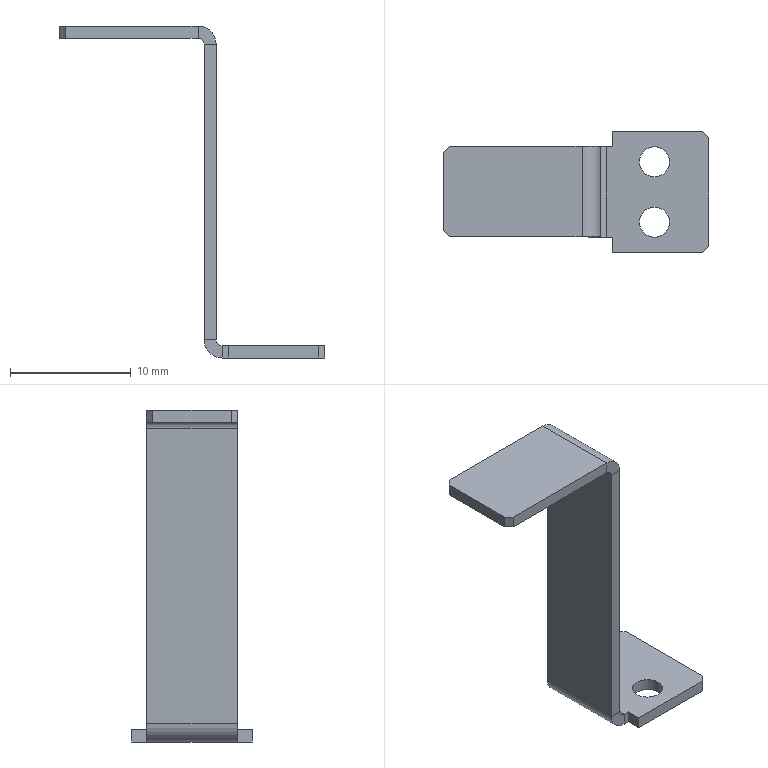Part | NX | 1 solid | 32 faces | box 22 x 10 x 27.5 mm | volume 366.994 mm3 | plane 26 | cylinder 6 | commonest cylinder face diameters 1 x2 2.5 x2 3 x2
STEP:
#1=CARTESIAN_POINT('',(-1.,3.75,0.5));
#2=VERTEX_POINT('',#1);
#3=CARTESIAN_POINT('',(-1.,3.75,25.));
#4=VERTEX_POINT('',#3);
#5=CARTESIAN_POINT('',(-1.,3.75,0.));
#6=DIRECTION('',(0.,0.,1.));
#7=VECTOR('',#6,1000.);
#8=LINE('',#5,#7);
#9=EDGE_CURVE('',#2,#4,#8,.T.);
#10=ORIENTED_EDGE('',*,*,#9,.T.);
#11=CARTESIAN_POINT('',(0.,3.75,25.));
#12=VERTEX_POINT('',#11);
#13=CARTESIAN_POINT('',(-1.,3.75,25.));
#14=DIRECTION('',(1.,0.,0.));
#15=VECTOR('',#14,1000.);
#16=LINE('',#13,#15);
#17=EDGE_CURVE('',#4,#12,#16,.T.);
#18=ORIENTED_EDGE('',*,*,#17,.T.);
#19=CARTESIAN_POINT('',(0.,3.75,0.5));
#20=VERTEX_POINT('',#19);
#21=CARTESIAN_POINT('',(0.,3.75,0.));
#22=DIRECTION('',(0.,0.,1.));
#23=VECTOR('',#22,1000.);
#24=LINE('',#21,#23);
#25=EDGE_CURVE('',#20,#12,#24,.T.);
#26=ORIENTED_EDGE('',*,*,#25,.F.);
#27=CARTESIAN_POINT('',(0.,3.75,0.5));
#28=DIRECTION('',(-1.,0.,0.));
#29=VECTOR('',#28,1000.);
#30=LINE('',#27,#29);
#31=EDGE_CURVE('',#20,#2,#30,.T.);
#32=ORIENTED_EDGE('',*,*,#31,.T.);
#33=EDGE_LOOP('',(#10,#18,#26,#32));
#34=FACE_BOUND('',#33,.T.);
#35=CARTESIAN_POINT('',(0.5,3.75,-1.));
#36=DIRECTION('',(0.,1.,0.));
#37=DIRECTION('',(0.,0.,1.));
#38=AXIS2_PLACEMENT_3D('',#35,#36,#37);
#39=PLANE('',#38);
#40=ADVANCED_FACE('',(#34),#39,.T.);
#41=CARTESIAN_POINT('',(-1.,-3.75,25.));
#42=VERTEX_POINT('',#41);
#43=CARTESIAN_POINT('',(-1.,3.75,25.));
#44=DIRECTION('',(0.,1.,0.));
#45=VECTOR('',#44,1000.);
#46=LINE('',#43,#45);
#47=EDGE_CURVE('',#4,#42,#46,.F.);
#48=ORIENTED_EDGE('',*,*,#47,.F.);
#49=ORIENTED_EDGE('',*,*,#9,.F.);
#50=CARTESIAN_POINT('',(-1.,-3.75,0.5));
#51=VERTEX_POINT('',#50);
#52=CARTESIAN_POINT('',(-1.,3.75,0.5));
#53=DIRECTION('',(0.,-1.,0.));
#54=VECTOR('',#53,1000.);
#55=LINE('',#52,#54);
#56=EDGE_CURVE('',#2,#51,#55,.T.);
#57=ORIENTED_EDGE('',*,*,#56,.T.);
#58=CARTESIAN_POINT('',(-1.,-3.75,0.));
#59=DIRECTION('',(0.,0.,1.));
#60=VECTOR('',#59,1000.);
#61=LINE('',#58,#60);
#62=EDGE_CURVE('',#51,#42,#61,.T.);
#63=ORIENTED_EDGE('',*,*,#62,.T.);
#64=EDGE_LOOP('',(#48,#49,#57,#63));
#65=FACE_BOUND('',#64,.T.);
#66=CARTESIAN_POINT('',(-1.,3.75,0.));
#67=DIRECTION('',(1.,0.,0.));
#68=DIRECTION('',(0.,0.,-1.));
#69=AXIS2_PLACEMENT_3D('',#66,#67,#68);
#70=PLANE('',#69);
#71=ADVANCED_FACE('',(#65),#70,.F.);
#72=ORIENTED_EDGE('',*,*,#25,.T.);
#73=CARTESIAN_POINT('',(0.,-3.75,25.));
#74=VERTEX_POINT('',#73);
#75=CARTESIAN_POINT('',(0.,3.75,25.));
#76=DIRECTION('',(0.,1.,0.));
#77=VECTOR('',#76,1000.);
#78=LINE('',#75,#77);
#79=EDGE_CURVE('',#12,#74,#78,.F.);
#80=ORIENTED_EDGE('',*,*,#79,.T.);
#81=CARTESIAN_POINT('',(0.,-3.75,0.5));
#82=VERTEX_POINT('',#81);
#83=CARTESIAN_POINT('',(0.,-3.75,0.));
#84=DIRECTION('',(0.,0.,1.));
#85=VECTOR('',#84,1000.);
#86=LINE('',#83,#85);
#87=EDGE_CURVE('',#82,#74,#86,.T.);
#88=ORIENTED_EDGE('',*,*,#87,.F.);
#89=CARTESIAN_POINT('',(0.,3.75,0.5));
#90=DIRECTION('',(0.,-1.,0.));
#91=VECTOR('',#90,1000.);
#92=LINE('',#89,#91);
#93=EDGE_CURVE('',#20,#82,#92,.T.);
#94=ORIENTED_EDGE('',*,*,#93,.F.);
#95=EDGE_LOOP('',(#72,#80,#88,#94));
#96=FACE_BOUND('',#95,.T.);
#97=CARTESIAN_POINT('',(0.,3.75,0.));
#98=DIRECTION('',(1.,0.,0.));
#99=DIRECTION('',(0.,0.,-1.));
#100=AXIS2_PLACEMENT_3D('',#97,#98,#99);
#101=PLANE('',#100);
#102=ADVANCED_FACE('',(#96),#101,.T.);
#103=ORIENTED_EDGE('',*,*,#31,.F.);
#104=CARTESIAN_POINT('',(0.5,3.75,0.));
#105=VERTEX_POINT('',#104);
#106=CARTESIAN_POINT('',(0.5,3.75,0.5));
#107=DIRECTION('',(0.,-1.,0.));
#108=DIRECTION('',(0.,0.,-1.));
#109=AXIS2_PLACEMENT_3D('',#106,#107,#108);
#110=CIRCLE('',#109,0.5);
#111=EDGE_CURVE('',#105,#20,#110,.F.);
#112=ORIENTED_EDGE('',*,*,#111,.F.);
#113=CARTESIAN_POINT('',(0.5,3.75,-1.));
#114=VERTEX_POINT('',#113);
#115=CARTESIAN_POINT('',(0.5,3.75,-1.));
#116=DIRECTION('',(0.,0.,1.));
#117=VECTOR('',#116,1000.);
#118=LINE('',#115,#117);
#119=EDGE_CURVE('',#114,#105,#118,.T.);
#120=ORIENTED_EDGE('',*,*,#119,.F.);
#121=CARTESIAN_POINT('',(0.5,3.75,0.5));
#122=DIRECTION('',(0.,1.,0.));
#123=DIRECTION('',(1.,0.,0.));
#124=AXIS2_PLACEMENT_3D('',#121,#122,#123);
#125=CIRCLE('',#124,1.5);
#126=EDGE_CURVE('',#114,#2,#125,.T.);
#127=ORIENTED_EDGE('',*,*,#126,.T.);
#128=EDGE_LOOP('',(#103,#112,#120,#127));
#129=FACE_BOUND('',#128,.T.);
#130=CARTESIAN_POINT('',(0.,3.75,0.5));
#131=DIRECTION('',(0.,1.,0.));
#132=DIRECTION('',(0.,0.,1.));
#133=AXIS2_PLACEMENT_3D('',#130,#131,#132);
#134=PLANE('',#133);
#135=ADVANCED_FACE('',(#129),#134,.T.);
#136=CARTESIAN_POINT('',(0.5,-3.75,0.));
#137=VERTEX_POINT('',#136);
#138=CARTESIAN_POINT('',(0.5,-3.75,-1.));
#139=VERTEX_POINT('',#138);
#140=CARTESIAN_POINT('',(0.5,-3.75,0.));
#141=DIRECTION('',(0.,0.,-1.));
#142=VECTOR('',#141,1000.);
#143=LINE('',#140,#142);
#144=EDGE_CURVE('',#137,#139,#143,.T.);
#145=ORIENTED_EDGE('',*,*,#144,.F.);
#146=CARTESIAN_POINT('',(0.5,-3.75,0.5));
#147=DIRECTION('',(0.,-1.,0.));
#148=DIRECTION('',(0.,0.,-1.));
#149=AXIS2_PLACEMENT_3D('',#146,#147,#148);
#150=CIRCLE('',#149,0.5);
#151=EDGE_CURVE('',#137,#82,#150,.F.);
#152=ORIENTED_EDGE('',*,*,#151,.T.);
#153=CARTESIAN_POINT('',(-1.,-3.75,0.5));
#154=DIRECTION('',(1.,0.,0.));
#155=VECTOR('',#154,1000.);
#156=LINE('',#153,#155);
#157=EDGE_CURVE('',#51,#82,#156,.T.);
#158=ORIENTED_EDGE('',*,*,#157,.F.);
#159=CARTESIAN_POINT('',(0.5,-3.75,0.5));
#160=DIRECTION('',(0.,1.,0.));
#161=DIRECTION('',(1.,0.,0.));
#162=AXIS2_PLACEMENT_3D('',#159,#160,#161);
#163=CIRCLE('',#162,1.5);
#164=EDGE_CURVE('',#139,#51,#163,.T.);
#165=ORIENTED_EDGE('',*,*,#164,.F.);
#166=EDGE_LOOP('',(#145,#152,#158,#165));
#167=FACE_BOUND('',#166,.T.);
#168=CARTESIAN_POINT('',(0.5,-3.75,0.));
#169=DIRECTION('',(0.,-1.,0.));
#170=DIRECTION('',(0.,0.,-1.));
#171=AXIS2_PLACEMENT_3D('',#168,#169,#170);
#172=PLANE('',#171);
#173=ADVANCED_FACE('',(#167),#172,.T.);
#174=CARTESIAN_POINT('',(1.,-3.75,0.));
#175=VERTEX_POINT('',#174);
#176=CARTESIAN_POINT('',(1.,-3.75,-1.));
#177=VERTEX_POINT('',#176);
#178=CARTESIAN_POINT('',(1.,-3.75,0.5));
#179=DIRECTION('',(0.,0.,-1.));
#180=VECTOR('',#179,1000.);
#181=LINE('',#178,#180);
#182=EDGE_CURVE('',#175,#177,#181,.T.);
#183=ORIENTED_EDGE('',*,*,#182,.F.);
#184=CARTESIAN_POINT('',(9.,-3.75,0.));
#185=DIRECTION('',(-1.,0.,0.));
#186=VECTOR('',#185,1000.);
#187=LINE('',#184,#186);
#188=EDGE_CURVE('',#175,#137,#187,.T.);
#189=ORIENTED_EDGE('',*,*,#188,.T.);
#190=ORIENTED_EDGE('',*,*,#144,.T.);
#191=CARTESIAN_POINT('',(9.,-3.75,-1.));
#192=DIRECTION('',(-1.,0.,0.));
#193=VECTOR('',#192,1000.);
#194=LINE('',#191,#193);
#195=EDGE_CURVE('',#177,#139,#194,.T.);
#196=ORIENTED_EDGE('',*,*,#195,.F.);
#197=EDGE_LOOP('',(#183,#189,#190,#196));
#198=FACE_BOUND('',#197,.T.);
#199=CARTESIAN_POINT('',(-1.,-3.75,0.5));
#200=DIRECTION('',(0.,-1.,0.));
#201=DIRECTION('',(0.,0.,-1.));
#202=AXIS2_PLACEMENT_3D('',#199,#200,#201);
#203=PLANE('',#202);
#204=ADVANCED_FACE('',(#198),#203,.T.);
#205=ORIENTED_EDGE('',*,*,#151,.F.);
#206=CARTESIAN_POINT('',(0.5,3.75,0.));
#207=DIRECTION('',(0.,-1.,0.));
#208=VECTOR('',#207,1000.);
#209=LINE('',#206,#208);
#210=EDGE_CURVE('',#105,#137,#209,.T.);
#211=ORIENTED_EDGE('',*,*,#210,.F.);
#212=ORIENTED_EDGE('',*,*,#111,.T.);
#213=ORIENTED_EDGE('',*,*,#93,.T.);
#214=EDGE_LOOP('',(#205,#211,#212,#213));
#215=FACE_BOUND('',#214,.T.);
#216=CARTESIAN_POINT('',(0.5,3.75,0.5));
#217=DIRECTION('',(0.,-1.,0.));
#218=DIRECTION('',(0.,0.,-1.));
#219=AXIS2_PLACEMENT_3D('',#216,#217,#218);
#220=CYLINDRICAL_SURFACE('',#219,0.5);
#221=ADVANCED_FACE('',(#215),#220,.F.);
#222=CARTESIAN_POINT('',(5.75,2.5,0.));
#223=VERTEX_POINT('',#222);
#224=CARTESIAN_POINT('',(4.5,2.5,0.));
#225=DIRECTION('',(0.,0.,1.));
#226=DIRECTION('',(1.,0.,0.));
#227=AXIS2_PLACEMENT_3D('',#224,#225,#226);
#228=CIRCLE('',#227,1.25);
#229=EDGE_CURVE('',#223,#223,#228,.T.);
#230=ORIENTED_EDGE('',*,*,#229,.F.);
#231=EDGE_LOOP('',(#230));
#232=FACE_BOUND('',#231,.T.);
#233=CARTESIAN_POINT('',(5.75,-2.5,0.));
#234=VERTEX_POINT('',#233);
#235=CARTESIAN_POINT('',(4.5,-2.5,0.));
#236=DIRECTION('',(0.,0.,1.));
#237=DIRECTION('',(1.,0.,0.));
#238=AXIS2_PLACEMENT_3D('',#235,#236,#237);
#239=CIRCLE('',#238,1.25);
#240=EDGE_CURVE('',#234,#234,#239,.T.);
#241=ORIENTED_EDGE('',*,*,#240,.F.);
#242=EDGE_LOOP('',(#241));
#243=FACE_BOUND('',#242,.T.);
#244=CARTESIAN_POINT('',(8.5,-5.,0.));
#245=VERTEX_POINT('',#244);
#246=CARTESIAN_POINT('',(1.,-5.,0.));
#247=VERTEX_POINT('',#246);
#248=CARTESIAN_POINT('',(9.,-5.,0.));
#249=DIRECTION('',(-1.,0.,0.));
#250=VECTOR('',#249,1000.);
#251=LINE('',#248,#250);
#252=EDGE_CURVE('',#245,#247,#251,.T.);
#253=ORIENTED_EDGE('',*,*,#252,.F.);
#254=CARTESIAN_POINT('',(9.,-4.5,0.));
#255=VERTEX_POINT('',#254);
#256=CARTESIAN_POINT('',(13.125,-0.375,0.));
#257=DIRECTION('',(-0.7071,-0.7071,0.));
#258=VECTOR('',#257,1000.);
#259=LINE('',#256,#258);
#260=EDGE_CURVE('',#245,#255,#259,.F.);
#261=ORIENTED_EDGE('',*,*,#260,.T.);
#262=CARTESIAN_POINT('',(9.,4.5,0.));
#263=VERTEX_POINT('',#262);
#264=CARTESIAN_POINT('',(9.,3.75,0.));
#265=DIRECTION('',(0.,-1.,0.));
#266=VECTOR('',#265,1000.);
#267=LINE('',#264,#266);
#268=EDGE_CURVE('',#263,#255,#267,.T.);
#269=ORIENTED_EDGE('',*,*,#268,.F.);
#270=CARTESIAN_POINT('',(8.5,5.,0.));
#271=VERTEX_POINT('',#270);
#272=CARTESIAN_POINT('',(9.375,4.125,0.));
#273=DIRECTION('',(0.7071,-0.7071,0.));
#274=VECTOR('',#273,1000.);
#275=LINE('',#272,#274);
#276=EDGE_CURVE('',#263,#271,#275,.F.);
#277=ORIENTED_EDGE('',*,*,#276,.T.);
#278=CARTESIAN_POINT('',(1.,5.,0.));
#279=VERTEX_POINT('',#278);
#280=CARTESIAN_POINT('',(9.,5.,0.));
#281=DIRECTION('',(1.,0.,0.));
#282=VECTOR('',#281,1000.);
#283=LINE('',#280,#282);
#284=EDGE_CURVE('',#279,#271,#283,.T.);
#285=ORIENTED_EDGE('',*,*,#284,.F.);
#286=CARTESIAN_POINT('',(1.,3.75,0.));
#287=VERTEX_POINT('',#286);
#288=CARTESIAN_POINT('',(1.,5.,0.));
#289=DIRECTION('',(0.,1.,0.));
#290=VECTOR('',#289,1000.);
#291=LINE('',#288,#290);
#292=EDGE_CURVE('',#287,#279,#291,.T.);
#293=ORIENTED_EDGE('',*,*,#292,.F.);
#294=CARTESIAN_POINT('',(9.,3.75,0.));
#295=DIRECTION('',(-1.,0.,0.));
#296=VECTOR('',#295,1000.);
#297=LINE('',#294,#296);
#298=EDGE_CURVE('',#287,#105,#297,.T.);
#299=ORIENTED_EDGE('',*,*,#298,.T.);
#300=ORIENTED_EDGE('',*,*,#210,.T.);
#301=ORIENTED_EDGE('',*,*,#188,.F.);
#302=CARTESIAN_POINT('',(1.,5.,0.));
#303=DIRECTION('',(0.,1.,0.));
#304=VECTOR('',#303,1000.);
#305=LINE('',#302,#304);
#306=EDGE_CURVE('',#247,#175,#305,.T.);
#307=ORIENTED_EDGE('',*,*,#306,.F.);
#308=EDGE_LOOP('',(#253,#261,#269,#277,#285,#293,#299,#300,#301,#307));
#309=FACE_BOUND('',#308,.T.);
#310=CARTESIAN_POINT('',(9.,3.75,0.));
#311=DIRECTION('',(0.,0.,1.));
#312=DIRECTION('',(1.,0.,0.));
#313=AXIS2_PLACEMENT_3D('',#310,#311,#312);
#314=PLANE('',#313);
#315=ADVANCED_FACE('',(#232,#243,#309),#314,.T.);
#316=ORIENTED_EDGE('',*,*,#268,.T.);
#317=CARTESIAN_POINT('',(9.,-4.5,-1.));
#318=VERTEX_POINT('',#317);
#319=CARTESIAN_POINT('',(9.,-4.5,-1.));
#320=DIRECTION('',(0.,0.,-1.));
#321=VECTOR('',#320,1000.);
#322=LINE('',#319,#321);
#323=EDGE_CURVE('',#255,#318,#322,.T.);
#324=ORIENTED_EDGE('',*,*,#323,.T.);
#325=CARTESIAN_POINT('',(9.,4.5,-1.));
#326=VERTEX_POINT('',#325);
#327=CARTESIAN_POINT('',(9.,3.75,-1.));
#328=DIRECTION('',(0.,-1.,0.));
#329=VECTOR('',#328,1000.);
#330=LINE('',#327,#329);
#331=EDGE_CURVE('',#326,#318,#330,.T.);
#332=ORIENTED_EDGE('',*,*,#331,.F.);
#333=CARTESIAN_POINT('',(9.,4.5,-1.));
#334=DIRECTION('',(0.,0.,1.));
#335=VECTOR('',#334,1000.);
#336=LINE('',#333,#335);
#337=EDGE_CURVE('',#326,#263,#336,.T.);
#338=ORIENTED_EDGE('',*,*,#337,.T.);
#339=EDGE_LOOP('',(#316,#324,#332,#338));
#340=FACE_BOUND('',#339,.T.);
#341=CARTESIAN_POINT('',(9.,3.75,-1.));
#342=DIRECTION('',(1.,0.,0.));
#343=DIRECTION('',(0.,0.,-1.));
#344=AXIS2_PLACEMENT_3D('',#341,#342,#343);
#345=PLANE('',#344);
#346=ADVANCED_FACE('',(#340),#345,.T.);
#347=CARTESIAN_POINT('',(5.75,2.5,-1.));
#348=VERTEX_POINT('',#347);
#349=CARTESIAN_POINT('',(4.5,2.5,-1.));
#350=DIRECTION('',(0.,0.,1.));
#351=DIRECTION('',(1.,0.,0.));
#352=AXIS2_PLACEMENT_3D('',#349,#350,#351);
#353=CIRCLE('',#352,1.25);
#354=EDGE_CURVE('',#348,#348,#353,.T.);
#355=ORIENTED_EDGE('',*,*,#354,.T.);
#356=EDGE_LOOP('',(#355));
#357=FACE_BOUND('',#356,.T.);
#358=CARTESIAN_POINT('',(5.75,-2.5,-1.));
#359=VERTEX_POINT('',#358);
#360=CARTESIAN_POINT('',(4.5,-2.5,-1.));
#361=DIRECTION('',(0.,0.,1.));
#362=DIRECTION('',(1.,0.,0.));
#363=AXIS2_PLACEMENT_3D('',#360,#361,#362);
#364=CIRCLE('',#363,1.25);
#365=EDGE_CURVE('',#359,#359,#364,.T.);
#366=ORIENTED_EDGE('',*,*,#365,.T.);
#367=EDGE_LOOP('',(#366));
#368=FACE_BOUND('',#367,.T.);
#369=ORIENTED_EDGE('',*,*,#331,.T.);
#370=CARTESIAN_POINT('',(8.5,-5.,-1.));
#371=VERTEX_POINT('',#370);
#372=CARTESIAN_POINT('',(9.,-4.5,-1.));
#373=DIRECTION('',(0.7071,0.7071,0.));
#374=VECTOR('',#373,1000.);
#375=LINE('',#372,#374);
#376=EDGE_CURVE('',#318,#371,#375,.F.);
#377=ORIENTED_EDGE('',*,*,#376,.T.);
#378=CARTESIAN_POINT('',(1.,-5.,-1.));
#379=VERTEX_POINT('',#378);
#380=CARTESIAN_POINT('',(9.,-5.,-1.));
#381=DIRECTION('',(-1.,0.,0.));
#382=VECTOR('',#381,1000.);
#383=LINE('',#380,#382);
#384=EDGE_CURVE('',#371,#379,#383,.T.);
#385=ORIENTED_EDGE('',*,*,#384,.T.);
#386=CARTESIAN_POINT('',(1.,5.,-1.));
#387=DIRECTION('',(0.,1.,0.));
#388=VECTOR('',#387,1000.);
#389=LINE('',#386,#388);
#390=EDGE_CURVE('',#379,#177,#389,.T.);
#391=ORIENTED_EDGE('',*,*,#390,.T.);
#392=ORIENTED_EDGE('',*,*,#195,.T.);
#393=CARTESIAN_POINT('',(0.5,3.75,-1.));
#394=DIRECTION('',(0.,-1.,0.));
#395=VECTOR('',#394,1000.);
#396=LINE('',#393,#395);
#397=EDGE_CURVE('',#114,#139,#396,.T.);
#398=ORIENTED_EDGE('',*,*,#397,.F.);
#399=CARTESIAN_POINT('',(1.,3.75,-1.));
#400=VERTEX_POINT('',#399);
#401=CARTESIAN_POINT('',(9.,3.75,-1.));
#402=DIRECTION('',(-1.,0.,0.));
#403=VECTOR('',#402,1000.);
#404=LINE('',#401,#403);
#405=EDGE_CURVE('',#400,#114,#404,.T.);
#406=ORIENTED_EDGE('',*,*,#405,.F.);
#407=CARTESIAN_POINT('',(1.,5.,-1.));
#408=VERTEX_POINT('',#407);
#409=CARTESIAN_POINT('',(1.,5.,-1.));
#410=DIRECTION('',(0.,1.,0.));
#411=VECTOR('',#410,1000.);
#412=LINE('',#409,#411);
#413=EDGE_CURVE('',#400,#408,#412,.T.);
#414=ORIENTED_EDGE('',*,*,#413,.T.);
#415=CARTESIAN_POINT('',(8.5,5.,-1.));
#416=VERTEX_POINT('',#415);
#417=CARTESIAN_POINT('',(9.,5.,-1.));
#418=DIRECTION('',(1.,0.,0.));
#419=VECTOR('',#418,1000.);
#420=LINE('',#417,#419);
#421=EDGE_CURVE('',#408,#416,#420,.T.);
#422=ORIENTED_EDGE('',*,*,#421,.T.);
#423=CARTESIAN_POINT('',(8.5,5.,-1.));
#424=DIRECTION('',(-0.7071,0.7071,0.));
#425=VECTOR('',#424,1000.);
#426=LINE('',#423,#425);
#427=EDGE_CURVE('',#416,#326,#426,.F.);
#428=ORIENTED_EDGE('',*,*,#427,.T.);
#429=EDGE_LOOP('',(#369,#377,#385,#391,#392,#398,#406,#414,#422,#428));
#430=FACE_BOUND('',#429,.T.);
#431=CARTESIAN_POINT('',(9.,3.75,-1.));
#432=DIRECTION('',(0.,0.,1.));
#433=DIRECTION('',(1.,0.,0.));
#434=AXIS2_PLACEMENT_3D('',#431,#432,#433);
#435=PLANE('',#434);
#436=ADVANCED_FACE('',(#357,#368,#430),#435,.F.);
#437=ORIENTED_EDGE('',*,*,#164,.T.);
#438=ORIENTED_EDGE('',*,*,#56,.F.);
#439=ORIENTED_EDGE('',*,*,#126,.F.);
#440=ORIENTED_EDGE('',*,*,#397,.T.);
#441=EDGE_LOOP('',(#437,#438,#439,#440));
#442=FACE_BOUND('',#441,.T.);
#443=CARTESIAN_POINT('',(0.5,3.75,0.5));
#444=DIRECTION('',(0.,-1.,0.));
#445=DIRECTION('',(0.,0.,-1.));
#446=AXIS2_PLACEMENT_3D('',#443,#444,#445);
#447=CYLINDRICAL_SURFACE('',#446,1.5);
#448=ADVANCED_FACE('',(#442),#447,.T.);
#449=ORIENTED_EDGE('',*,*,#298,.F.);
#450=CARTESIAN_POINT('',(1.,3.75,0.5));
#451=DIRECTION('',(0.,0.,-1.));
#452=VECTOR('',#451,1000.);
#453=LINE('',#450,#452);
#454=EDGE_CURVE('',#287,#400,#453,.T.);
#455=ORIENTED_EDGE('',*,*,#454,.T.);
#456=ORIENTED_EDGE('',*,*,#405,.T.);
#457=ORIENTED_EDGE('',*,*,#119,.T.);
#458=EDGE_LOOP('',(#449,#455,#456,#457));
#459=FACE_BOUND('',#458,.T.);
#460=CARTESIAN_POINT('',(0.5,3.75,0.5));
#461=DIRECTION('',(0.,-1.,0.));
#462=DIRECTION('',(-1.,0.,0.));
#463=AXIS2_PLACEMENT_3D('',#460,#461,#462);
#464=PLANE('',#463);
#465=ADVANCED_FACE('',(#459),#464,.F.);
#466=CARTESIAN_POINT('',(-1.,-3.75,25.));
#467=DIRECTION('',(1.,0.,0.));
#468=VECTOR('',#467,1000.);
#469=LINE('',#466,#468);
#470=EDGE_CURVE('',#42,#74,#469,.T.);
#471=ORIENTED_EDGE('',*,*,#470,.F.);
#472=ORIENTED_EDGE('',*,*,#62,.F.);
#473=ORIENTED_EDGE('',*,*,#157,.T.);
#474=ORIENTED_EDGE('',*,*,#87,.T.);
#475=EDGE_LOOP('',(#471,#472,#473,#474));
#476=FACE_BOUND('',#475,.T.);
#477=CARTESIAN_POINT('',(0.5,-3.75,0.5));
#478=DIRECTION('',(0.,-1.,0.));
#479=DIRECTION('',(-1.,0.,0.));
#480=AXIS2_PLACEMENT_3D('',#477,#478,#479);
#481=PLANE('',#480);
#482=ADVANCED_FACE('',(#476),#481,.T.);
#483=CARTESIAN_POINT('',(-1.5,-3.75,25.5));
#484=VERTEX_POINT('',#483);
#485=CARTESIAN_POINT('',(-1.5,-3.75,26.5));
#486=VERTEX_POINT('',#485);
#487=CARTESIAN_POINT('',(-1.5,-3.75,25.5));
#488=DIRECTION('',(0.,0.,1.));
#489=VECTOR('',#488,1000.);
#490=LINE('',#487,#489);
#491=EDGE_CURVE('',#484,#486,#490,.T.);
#492=ORIENTED_EDGE('',*,*,#491,.F.);
#493=CARTESIAN_POINT('',(-1.5,-3.75,25.));
#494=DIRECTION('',(0.,1.,0.));
#495=DIRECTION('',(0.,0.,1.));
#496=AXIS2_PLACEMENT_3D('',#493,#494,#495);
#497=CIRCLE('',#496,0.5);
#498=EDGE_CURVE('',#42,#484,#497,.F.);
#499=ORIENTED_EDGE('',*,*,#498,.F.);
#500=ORIENTED_EDGE('',*,*,#470,.T.);
#501=CARTESIAN_POINT('',(-1.5,-3.75,25.));
#502=DIRECTION('',(0.,1.,0.));
#503=DIRECTION('',(0.,0.,1.));
#504=AXIS2_PLACEMENT_3D('',#501,#502,#503);
#505=CIRCLE('',#504,1.5);
#506=EDGE_CURVE('',#74,#486,#505,.F.);
#507=ORIENTED_EDGE('',*,*,#506,.T.);
#508=EDGE_LOOP('',(#492,#499,#500,#507));
#509=FACE_BOUND('',#508,.T.);
#510=CARTESIAN_POINT('',(-1.5,-3.75,25.));
#511=DIRECTION('',(0.,-1.,0.));
#512=DIRECTION('',(0.,0.,-1.));
#513=AXIS2_PLACEMENT_3D('',#510,#511,#512);
#514=PLANE('',#513);
#515=ADVANCED_FACE('',(#509),#514,.T.);
#516=CARTESIAN_POINT('',(-1.5,3.75,25.5));
#517=VERTEX_POINT('',#516);
#518=CARTESIAN_POINT('',(-1.5,3.75,25.));
#519=DIRECTION('',(0.,1.,0.));
#520=DIRECTION('',(0.,0.,1.));
#521=AXIS2_PLACEMENT_3D('',#518,#519,#520);
#522=CIRCLE('',#521,0.5);
#523=EDGE_CURVE('',#517,#4,#522,.T.);
#524=ORIENTED_EDGE('',*,*,#523,.F.);
#525=CARTESIAN_POINT('',(-1.5,3.75,26.5));
#526=VERTEX_POINT('',#525);
#527=CARTESIAN_POINT('',(-1.5,3.75,25.5));
#528=DIRECTION('',(0.,0.,1.));
#529=VECTOR('',#528,1000.);
#530=LINE('',#527,#529);
#531=EDGE_CURVE('',#517,#526,#530,.T.);
#532=ORIENTED_EDGE('',*,*,#531,.T.);
#533=CARTESIAN_POINT('',(-1.5,3.75,25.));
#534=DIRECTION('',(0.,1.,0.));
#535=DIRECTION('',(0.,0.,1.));
#536=AXIS2_PLACEMENT_3D('',#533,#534,#535);
#537=CIRCLE('',#536,1.5);
#538=EDGE_CURVE('',#526,#12,#537,.T.);
#539=ORIENTED_EDGE('',*,*,#538,.T.);
#540=ORIENTED_EDGE('',*,*,#17,.F.);
#541=EDGE_LOOP('',(#524,#532,#539,#540));
#542=FACE_BOUND('',#541,.T.);
#543=CARTESIAN_POINT('',(-1.5,3.75,25.));
#544=DIRECTION('',(0.,-1.,0.));
#545=DIRECTION('',(0.,0.,-1.));
#546=AXIS2_PLACEMENT_3D('',#543,#544,#545);
#547=PLANE('',#546);
#548=ADVANCED_FACE('',(#542),#547,.F.);
#549=ORIENTED_EDGE('',*,*,#79,.F.);
#550=ORIENTED_EDGE('',*,*,#538,.F.);
#551=CARTESIAN_POINT('',(-1.5,0.,26.5));
#552=DIRECTION('',(0.,-1.,0.));
#553=VECTOR('',#552,1000.);
#554=LINE('',#551,#553);
#555=EDGE_CURVE('',#526,#486,#554,.T.);
#556=ORIENTED_EDGE('',*,*,#555,.T.);
#557=ORIENTED_EDGE('',*,*,#506,.F.);
#558=EDGE_LOOP('',(#549,#550,#556,#557));
#559=FACE_BOUND('',#558,.T.);
#560=CARTESIAN_POINT('',(-1.5,3.75,25.));
#561=DIRECTION('',(0.,1.,0.));
#562=DIRECTION('',(0.,0.,1.));
#563=AXIS2_PLACEMENT_3D('',#560,#561,#562);
#564=CYLINDRICAL_SURFACE('',#563,1.5);
#565=ADVANCED_FACE('',(#559),#564,.T.);
#566=ORIENTED_EDGE('',*,*,#47,.T.);
#567=ORIENTED_EDGE('',*,*,#498,.T.);
#568=CARTESIAN_POINT('',(-1.5,-3.75,25.5));
#569=DIRECTION('',(0.,1.,0.));
#570=VECTOR('',#569,1000.);
#571=LINE('',#568,#570);
#572=EDGE_CURVE('',#484,#517,#571,.T.);
#573=ORIENTED_EDGE('',*,*,#572,.T.);
#574=ORIENTED_EDGE('',*,*,#523,.T.);
#575=EDGE_LOOP('',(#566,#567,#573,#574));
#576=FACE_BOUND('',#575,.T.);
#577=CARTESIAN_POINT('',(-1.5,3.75,25.));
#578=DIRECTION('',(0.,1.,0.));
#579=DIRECTION('',(0.,0.,1.));
#580=AXIS2_PLACEMENT_3D('',#577,#578,#579);
#581=CYLINDRICAL_SURFACE('',#580,0.5);
#582=ADVANCED_FACE('',(#576),#581,.F.);
#583=CARTESIAN_POINT('',(-12.5,3.75,25.5));
#584=VERTEX_POINT('',#583);
#585=CARTESIAN_POINT('',(-13.,3.75,25.5));
#586=DIRECTION('',(-1.,0.,0.));
#587=VECTOR('',#586,1000.);
#588=LINE('',#585,#587);
#589=EDGE_CURVE('',#517,#584,#588,.T.);
#590=ORIENTED_EDGE('',*,*,#589,.T.);
#591=CARTESIAN_POINT('',(-12.5,3.75,26.5));
#592=VERTEX_POINT('',#591);
#593=CARTESIAN_POINT('',(-12.5,3.75,26.5));
#594=DIRECTION('',(0.,0.,1.));
#595=VECTOR('',#594,1000.);
#596=LINE('',#593,#595);
#597=EDGE_CURVE('',#584,#592,#596,.T.);
#598=ORIENTED_EDGE('',*,*,#597,.T.);
#599=CARTESIAN_POINT('',(-13.,3.75,26.5));
#600=DIRECTION('',(-1.,0.,0.));
#601=VECTOR('',#600,1000.);
#602=LINE('',#599,#601);
#603=EDGE_CURVE('',#526,#592,#602,.T.);
#604=ORIENTED_EDGE('',*,*,#603,.F.);
#605=ORIENTED_EDGE('',*,*,#531,.F.);
#606=EDGE_LOOP('',(#590,#598,#604,#605));
#607=FACE_BOUND('',#606,.T.);
#608=CARTESIAN_POINT('',(-13.,3.75,26.5));
#609=DIRECTION('',(0.,-1.,0.));
#610=DIRECTION('',(1.,0.,0.));
#611=AXIS2_PLACEMENT_3D('',#608,#609,#610);
#612=PLANE('',#611);
#613=ADVANCED_FACE('',(#607),#612,.F.);
#614=CARTESIAN_POINT('',(-12.5,-3.75,26.5));
#615=VERTEX_POINT('',#614);
#616=CARTESIAN_POINT('',(-1.,-3.75,26.5));
#617=DIRECTION('',(1.,0.,0.));
#618=VECTOR('',#617,1000.);
#619=LINE('',#616,#618);
#620=EDGE_CURVE('',#615,#486,#619,.T.);
#621=ORIENTED_EDGE('',*,*,#620,.F.);
#622=CARTESIAN_POINT('',(-12.5,-3.75,25.5));
#623=VERTEX_POINT('',#622);
#624=CARTESIAN_POINT('',(-12.5,-3.75,26.5));
#625=DIRECTION('',(0.,0.,-1.));
#626=VECTOR('',#625,1000.);
#627=LINE('',#624,#626);
#628=EDGE_CURVE('',#615,#623,#627,.T.);
#629=ORIENTED_EDGE('',*,*,#628,.T.);
#630=CARTESIAN_POINT('',(-1.,-3.75,25.5));
#631=DIRECTION('',(1.,0.,0.));
#632=VECTOR('',#631,1000.);
#633=LINE('',#630,#632);
#634=EDGE_CURVE('',#623,#484,#633,.T.);
#635=ORIENTED_EDGE('',*,*,#634,.T.);
#636=ORIENTED_EDGE('',*,*,#491,.T.);
#637=EDGE_LOOP('',(#621,#629,#635,#636));
#638=FACE_BOUND('',#637,.T.);
#639=CARTESIAN_POINT('',(-1.,-3.75,26.5));
#640=DIRECTION('',(0.,1.,0.));
#641=DIRECTION('',(0.,0.,1.));
#642=AXIS2_PLACEMENT_3D('',#639,#640,#641);
#643=PLANE('',#642);
#644=ADVANCED_FACE('',(#638),#643,.F.);
#645=ORIENTED_EDGE('',*,*,#603,.T.);
#646=CARTESIAN_POINT('',(-13.,3.25,26.5));
#647=VERTEX_POINT('',#646);
#648=CARTESIAN_POINT('',(-13.,3.25,26.5));
#649=DIRECTION('',(0.7071,0.7071,0.));
#650=VECTOR('',#649,1000.);
#651=LINE('',#648,#650);
#652=EDGE_CURVE('',#592,#647,#651,.F.);
#653=ORIENTED_EDGE('',*,*,#652,.T.);
#654=CARTESIAN_POINT('',(-13.,-3.25,26.5));
#655=VERTEX_POINT('',#654);
#656=CARTESIAN_POINT('',(-13.,-3.75,26.5));
#657=DIRECTION('',(0.,-1.,0.));
#658=VECTOR('',#657,1000.);
#659=LINE('',#656,#658);
#660=EDGE_CURVE('',#647,#655,#659,.T.);
#661=ORIENTED_EDGE('',*,*,#660,.T.);
#662=CARTESIAN_POINT('',(-12.5,-3.75,26.5));
#663=DIRECTION('',(-0.7071,0.7071,0.));
#664=VECTOR('',#663,1000.);
#665=LINE('',#662,#664);
#666=EDGE_CURVE('',#655,#615,#665,.F.);
#667=ORIENTED_EDGE('',*,*,#666,.T.);
#668=ORIENTED_EDGE('',*,*,#620,.T.);
#669=ORIENTED_EDGE('',*,*,#555,.F.);
#670=EDGE_LOOP('',(#645,#653,#661,#667,#668,#669));
#671=FACE_BOUND('',#670,.T.);
#672=CARTESIAN_POINT('',(0.,0.,26.5));
#673=DIRECTION('',(0.,0.,-1.));
#674=DIRECTION('',(-1.,0.,0.));
#675=AXIS2_PLACEMENT_3D('',#672,#673,#674);
#676=PLANE('',#675);
#677=ADVANCED_FACE('',(#671),#676,.F.);
#678=CARTESIAN_POINT('',(-13.,3.25,25.5));
#679=VERTEX_POINT('',#678);
#680=CARTESIAN_POINT('',(-13.,-3.25,25.5));
#681=VERTEX_POINT('',#680);
#682=CARTESIAN_POINT('',(-13.,-3.75,25.5));
#683=DIRECTION('',(0.,-1.,0.));
#684=VECTOR('',#683,1000.);
#685=LINE('',#682,#684);
#686=EDGE_CURVE('',#679,#681,#685,.T.);
#687=ORIENTED_EDGE('',*,*,#686,.F.);
#688=CARTESIAN_POINT('',(-8.125,8.125,25.5));
#689=DIRECTION('',(-0.7071,-0.7071,0.));
#690=VECTOR('',#689,1000.);
#691=LINE('',#688,#690);
#692=EDGE_CURVE('',#679,#584,#691,.F.);
#693=ORIENTED_EDGE('',*,*,#692,.T.);
#694=ORIENTED_EDGE('',*,*,#589,.F.);
#695=ORIENTED_EDGE('',*,*,#572,.F.);
#696=ORIENTED_EDGE('',*,*,#634,.F.);
#697=CARTESIAN_POINT('',(-8.125,-8.125,25.5));
#698=DIRECTION('',(0.7071,-0.7071,0.));
#699=VECTOR('',#698,1000.);
#700=LINE('',#697,#699);
#701=EDGE_CURVE('',#623,#681,#700,.F.);
#702=ORIENTED_EDGE('',*,*,#701,.T.);
#703=EDGE_LOOP('',(#687,#693,#694,#695,#696,#702));
#704=FACE_BOUND('',#703,.T.);
#705=CARTESIAN_POINT('',(0.,0.,25.5));
#706=DIRECTION('',(0.,0.,-1.));
#707=DIRECTION('',(-1.,0.,0.));
#708=AXIS2_PLACEMENT_3D('',#705,#706,#707);
#709=PLANE('',#708);
#710=ADVANCED_FACE('',(#704),#709,.T.);
#711=ORIENTED_EDGE('',*,*,#660,.F.);
#712=CARTESIAN_POINT('',(-13.,3.25,26.5));
#713=DIRECTION('',(0.,0.,-1.));
#714=VECTOR('',#713,1000.);
#715=LINE('',#712,#714);
#716=EDGE_CURVE('',#647,#679,#715,.T.);
#717=ORIENTED_EDGE('',*,*,#716,.T.);
#718=ORIENTED_EDGE('',*,*,#686,.T.);
#719=CARTESIAN_POINT('',(-13.,-3.25,26.5));
#720=DIRECTION('',(0.,0.,1.));
#721=VECTOR('',#720,1000.);
#722=LINE('',#719,#721);
#723=EDGE_CURVE('',#681,#655,#722,.T.);
#724=ORIENTED_EDGE('',*,*,#723,.T.);
#725=EDGE_LOOP('',(#711,#717,#718,#724));
#726=FACE_BOUND('',#725,.T.);
#727=CARTESIAN_POINT('',(-13.,-3.75,26.5));
#728=DIRECTION('',(1.,0.,0.));
#729=DIRECTION('',(0.,0.,-1.));
#730=AXIS2_PLACEMENT_3D('',#727,#728,#729);
#731=PLANE('',#730);
#732=ADVANCED_FACE('',(#726),#731,.F.);
#733=ORIENTED_EDGE('',*,*,#284,.T.);
#734=CARTESIAN_POINT('',(8.5,5.,0.));
#735=DIRECTION('',(0.,0.,-1.));
#736=VECTOR('',#735,1000.);
#737=LINE('',#734,#736);
#738=EDGE_CURVE('',#271,#416,#737,.T.);
#739=ORIENTED_EDGE('',*,*,#738,.T.);
#740=ORIENTED_EDGE('',*,*,#421,.F.);
#741=CARTESIAN_POINT('',(1.,5.,0.));
#742=DIRECTION('',(0.,0.,-1.));
#743=VECTOR('',#742,1000.);
#744=LINE('',#741,#743);
#745=EDGE_CURVE('',#279,#408,#744,.T.);
#746=ORIENTED_EDGE('',*,*,#745,.F.);
#747=EDGE_LOOP('',(#733,#739,#740,#746));
#748=FACE_BOUND('',#747,.T.);
#749=CARTESIAN_POINT('',(9.,5.,0.));
#750=DIRECTION('',(0.,1.,0.));
#751=DIRECTION('',(-1.,0.,0.));
#752=AXIS2_PLACEMENT_3D('',#749,#750,#751);
#753=PLANE('',#752);
#754=ADVANCED_FACE('',(#748),#753,.T.);
#755=ORIENTED_EDGE('',*,*,#454,.F.);
#756=ORIENTED_EDGE('',*,*,#292,.T.);
#757=ORIENTED_EDGE('',*,*,#745,.T.);
#758=ORIENTED_EDGE('',*,*,#413,.F.);
#759=EDGE_LOOP('',(#755,#756,#757,#758));
#760=FACE_BOUND('',#759,.T.);
#761=CARTESIAN_POINT('',(1.,5.,0.));
#762=DIRECTION('',(-1.,0.,0.));
#763=DIRECTION('',(0.,-1.,0.));
#764=AXIS2_PLACEMENT_3D('',#761,#762,#763);
#765=PLANE('',#764);
#766=ADVANCED_FACE('',(#760),#765,.T.);
#767=ORIENTED_EDGE('',*,*,#306,.T.);
#768=ORIENTED_EDGE('',*,*,#182,.T.);
#769=ORIENTED_EDGE('',*,*,#390,.F.);
#770=CARTESIAN_POINT('',(1.,-5.,0.));
#771=DIRECTION('',(0.,0.,-1.));
#772=VECTOR('',#771,1000.);
#773=LINE('',#770,#772);
#774=EDGE_CURVE('',#247,#379,#773,.T.);
#775=ORIENTED_EDGE('',*,*,#774,.F.);
#776=EDGE_LOOP('',(#767,#768,#769,#775));
#777=FACE_BOUND('',#776,.T.);
#778=CARTESIAN_POINT('',(1.,5.,0.));
#779=DIRECTION('',(-1.,0.,0.));
#780=DIRECTION('',(0.,-1.,0.));
#781=AXIS2_PLACEMENT_3D('',#778,#779,#780);
#782=PLANE('',#781);
#783=ADVANCED_FACE('',(#777),#782,.T.);
#784=ORIENTED_EDGE('',*,*,#384,.F.);
#785=CARTESIAN_POINT('',(8.5,-5.,0.));
#786=DIRECTION('',(0.,0.,1.));
#787=VECTOR('',#786,1000.);
#788=LINE('',#785,#787);
#789=EDGE_CURVE('',#371,#245,#788,.T.);
#790=ORIENTED_EDGE('',*,*,#789,.T.);
#791=ORIENTED_EDGE('',*,*,#252,.T.);
#792=ORIENTED_EDGE('',*,*,#774,.T.);
#793=EDGE_LOOP('',(#784,#790,#791,#792));
#794=FACE_BOUND('',#793,.T.);
#795=CARTESIAN_POINT('',(9.,-5.,0.));
#796=DIRECTION('',(0.,-1.,0.));
#797=DIRECTION('',(1.,0.,0.));
#798=AXIS2_PLACEMENT_3D('',#795,#796,#797);
#799=PLANE('',#798);
#800=ADVANCED_FACE('',(#794),#799,.T.);
#801=ORIENTED_EDGE('',*,*,#365,.F.);
#802=EDGE_LOOP('',(#801));
#803=FACE_BOUND('',#802,.T.);
#804=ORIENTED_EDGE('',*,*,#240,.T.);
#805=EDGE_LOOP('',(#804));
#806=FACE_BOUND('',#805,.T.);
#807=CARTESIAN_POINT('',(4.5,-2.5,0.));
#808=DIRECTION('',(0.,0.,1.));
#809=DIRECTION('',(1.,0.,0.));
#810=AXIS2_PLACEMENT_3D('',#807,#808,#809);
#811=CYLINDRICAL_SURFACE('',#810,1.25);
#812=ADVANCED_FACE('',(#803,#806),#811,.F.);
#813=ORIENTED_EDGE('',*,*,#354,.F.);
#814=EDGE_LOOP('',(#813));
#815=FACE_BOUND('',#814,.T.);
#816=ORIENTED_EDGE('',*,*,#229,.T.);
#817=EDGE_LOOP('',(#816));
#818=FACE_BOUND('',#817,.T.);
#819=CARTESIAN_POINT('',(4.5,2.5,0.));
#820=DIRECTION('',(0.,0.,1.));
#821=DIRECTION('',(1.,0.,0.));
#822=AXIS2_PLACEMENT_3D('',#819,#820,#821);
#823=CYLINDRICAL_SURFACE('',#822,1.25);
#824=ADVANCED_FACE('',(#815,#818),#823,.F.);
#825=ORIENTED_EDGE('',*,*,#652,.F.);
#826=ORIENTED_EDGE('',*,*,#597,.F.);
#827=ORIENTED_EDGE('',*,*,#692,.F.);
#828=ORIENTED_EDGE('',*,*,#716,.F.);
#829=EDGE_LOOP('',(#825,#826,#827,#828));
#830=FACE_BOUND('',#829,.T.);
#831=CARTESIAN_POINT('',(-13.,3.25,26.5));
#832=DIRECTION('',(0.7071,-0.7071,0.));
#833=DIRECTION('',(0.,0.,-1.));
#834=AXIS2_PLACEMENT_3D('',#831,#832,#833);
#835=PLANE('',#834);
#836=ADVANCED_FACE('',(#830),#835,.F.);
#837=ORIENTED_EDGE('',*,*,#666,.F.);
#838=ORIENTED_EDGE('',*,*,#723,.F.);
#839=ORIENTED_EDGE('',*,*,#701,.F.);
#840=ORIENTED_EDGE('',*,*,#628,.F.);
#841=EDGE_LOOP('',(#837,#838,#839,#840));
#842=FACE_BOUND('',#841,.T.);
#843=CARTESIAN_POINT('',(-12.5,-3.75,26.5));
#844=DIRECTION('',(0.7071,0.7071,0.));
#845=DIRECTION('',(0.,0.,-1.));
#846=AXIS2_PLACEMENT_3D('',#843,#844,#845);
#847=PLANE('',#846);
#848=ADVANCED_FACE('',(#842),#847,.F.);
#849=ORIENTED_EDGE('',*,*,#260,.F.);
#850=ORIENTED_EDGE('',*,*,#789,.F.);
#851=ORIENTED_EDGE('',*,*,#376,.F.);
#852=ORIENTED_EDGE('',*,*,#323,.F.);
#853=EDGE_LOOP('',(#849,#850,#851,#852));
#854=FACE_BOUND('',#853,.T.);
#855=CARTESIAN_POINT('',(9.,-4.5,-1.));
#856=DIRECTION('',(-0.7071,0.7071,0.));
#857=DIRECTION('',(0.,0.,-1.));
#858=AXIS2_PLACEMENT_3D('',#855,#856,#857);
#859=PLANE('',#858);
#860=ADVANCED_FACE('',(#854),#859,.F.);
#861=ORIENTED_EDGE('',*,*,#276,.F.);
#862=ORIENTED_EDGE('',*,*,#337,.F.);
#863=ORIENTED_EDGE('',*,*,#427,.F.);
#864=ORIENTED_EDGE('',*,*,#738,.F.);
#865=EDGE_LOOP('',(#861,#862,#863,#864));
#866=FACE_BOUND('',#865,.T.);
#867=CARTESIAN_POINT('',(8.5,5.,0.));
#868=DIRECTION('',(-0.7071,-0.7071,0.));
#869=DIRECTION('',(0.,0.,-1.));
#870=AXIS2_PLACEMENT_3D('',#867,#868,#869);
#871=PLANE('',#870);
#872=ADVANCED_FACE('',(#866),#871,.F.);
#873=CLOSED_SHELL('',(#40,#71,#102,#135,#173,#204,#221,#315,#346,#436,#448,#465,#482,#515,#548,#565,#582,#613,#644,#677,#710,#732,#754,#766,#783,#800,#812,#824,#836,#848,#860,#872));
#874=MANIFOLD_SOLID_BREP('',#873);
#875=(LENGTH_UNIT()NAMED_UNIT(*)SI_UNIT(.MILLI.,.METRE.));
#876=UNCERTAINTY_MEASURE_WITH_UNIT(LENGTH_MEASURE(0.00001),#875,'','');
#877=(NAMED_UNIT(*)PLANE_ANGLE_UNIT()SI_UNIT($,.RADIAN.));
#878=(NAMED_UNIT(*)SI_UNIT($,.STERADIAN.)SOLID_ANGLE_UNIT());
#879=(GEOMETRIC_REPRESENTATION_CONTEXT(3)GLOBAL_UNCERTAINTY_ASSIGNED_CONTEXT((#876))GLOBAL_UNIT_ASSIGNED_CONTEXT((#875,#877,#878))REPRESENTATION_CONTEXT('',''));
#880=ADVANCED_BREP_SHAPE_REPRESENTATION('',(#874),#879);